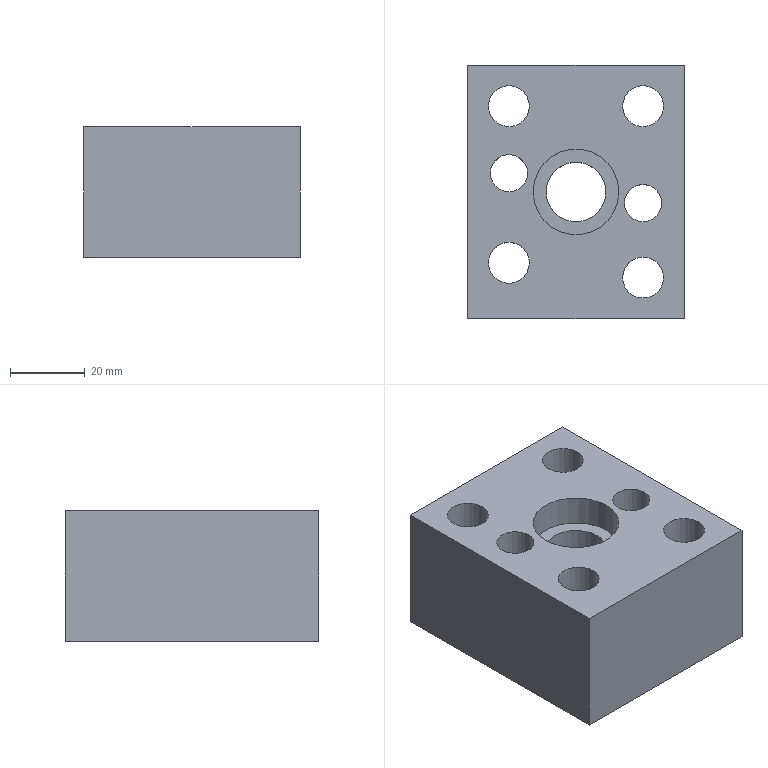Part | NX | features solid 2 | 1 solid | 27 faces | box 58 x 68 x 35 mm | volume 103779 mm3 | cylinder 14 | plane 13 | commonest cylinder face diameters 11 x6 17 x4 10 x2 16 x1 23 x1
STEP:
#1=CARTESIAN_POINT('',(1273.079,146.904,15.));
#2=VERTEX_POINT('',#1);
#3=CARTESIAN_POINT('',(1268.079,146.904,15.));
#4=DIRECTION('',(0.,0.,-1.));
#5=DIRECTION('',(1.,0.,0.));
#6=AXIS2_PLACEMENT_3D('',#3,#4,#5);
#7=CIRCLE('',#6,5.);
#8=EDGE_CURVE('',#2,#2,#7,.T.);
#9=ORIENTED_EDGE('',*,*,#8,.F.);
#10=EDGE_LOOP('',(#9));
#11=FACE_BOUND('',#10,.T.);
#12=CARTESIAN_POINT('',(1273.579,146.904,15.));
#13=VERTEX_POINT('',#12);
#14=CARTESIAN_POINT('',(1268.079,146.904,15.));
#15=DIRECTION('',(0.,0.,-1.));
#16=DIRECTION('',(1.,0.,0.));
#17=AXIS2_PLACEMENT_3D('',#14,#15,#16);
#18=CIRCLE('',#17,5.5);
#19=EDGE_CURVE('',#13,#13,#18,.T.);
#20=ORIENTED_EDGE('',*,*,#19,.T.);
#21=EDGE_LOOP('',(#20));
#22=FACE_BOUND('',#21,.T.);
#23=CARTESIAN_POINT('',(1266.894,137.78,15.));
#24=DIRECTION('',(0.,0.,1.));
#25=DIRECTION('',(1.,0.,0.));
#26=AXIS2_PLACEMENT_3D('',#23,#24,#25);
#27=PLANE('',#26);
#28=ADVANCED_FACE('',(#11,#22),#27,.F.);
#29=CARTESIAN_POINT('',(1273.079,146.904,40.));
#30=VERTEX_POINT('',#29);
#31=CARTESIAN_POINT('',(1268.079,146.904,40.));
#32=DIRECTION('',(0.,0.,-1.));
#33=DIRECTION('',(1.,0.,0.));
#34=AXIS2_PLACEMENT_3D('',#31,#32,#33);
#35=CIRCLE('',#34,5.);
#36=EDGE_CURVE('',#30,#30,#35,.T.);
#37=ORIENTED_EDGE('',*,*,#36,.F.);
#38=EDGE_LOOP('',(#37));
#39=FACE_BOUND('',#38,.T.);
#40=ORIENTED_EDGE('',*,*,#8,.T.);
#41=EDGE_LOOP('',(#40));
#42=FACE_BOUND('',#41,.T.);
#43=CARTESIAN_POINT('',(1268.079,146.904,40.));
#44=DIRECTION('',(0.,0.,1.));
#45=DIRECTION('',(1.,0.,0.));
#46=AXIS2_PLACEMENT_3D('',#43,#44,#45);
#47=CYLINDRICAL_SURFACE('',#46,5.);
#48=ADVANCED_FACE('',(#39,#42),#47,.F.);
#49=ORIENTED_EDGE('',*,*,#19,.F.);
#50=EDGE_LOOP('',(#49));
#51=FACE_BOUND('',#50,.T.);
#52=CARTESIAN_POINT('',(1273.579,146.904,5.));
#53=VERTEX_POINT('',#52);
#54=CARTESIAN_POINT('',(1268.079,146.904,5.));
#55=DIRECTION('',(0.,0.,-1.));
#56=DIRECTION('',(1.,0.,0.));
#57=AXIS2_PLACEMENT_3D('',#54,#55,#56);
#58=CIRCLE('',#57,5.5);
#59=EDGE_CURVE('',#53,#53,#58,.F.);
#60=ORIENTED_EDGE('',*,*,#59,.F.);
#61=EDGE_LOOP('',(#60));
#62=FACE_BOUND('',#61,.T.);
#63=CARTESIAN_POINT('',(1268.079,146.904,5.));
#64=DIRECTION('',(0.,0.,1.));
#65=DIRECTION('',(1.,0.,0.));
#66=AXIS2_PLACEMENT_3D('',#63,#64,#65);
#67=CYLINDRICAL_SURFACE('',#66,5.5);
#68=ADVANCED_FACE('',(#51,#62),#67,.F.);
#69=CARTESIAN_POINT('',(1298.579,118.904,17.));
#70=VERTEX_POINT('',#69);
#71=CARTESIAN_POINT('',(1304.079,118.904,17.));
#72=DIRECTION('',(0.,0.,1.));
#73=DIRECTION('',(-1.,0.,0.));
#74=AXIS2_PLACEMENT_3D('',#71,#72,#73);
#75=CIRCLE('',#74,5.5);
#76=EDGE_CURVE('',#70,#70,#75,.F.);
#77=ORIENTED_EDGE('',*,*,#76,.F.);
#78=EDGE_LOOP('',(#77));
#79=FACE_BOUND('',#78,.T.);
#80=CARTESIAN_POINT('',(1295.579,118.904,17.));
#81=VERTEX_POINT('',#80);
#82=CARTESIAN_POINT('',(1304.079,118.904,17.));
#83=DIRECTION('',(0.,0.,1.));
#84=DIRECTION('',(-1.,0.,0.));
#85=AXIS2_PLACEMENT_3D('',#82,#83,#84);
#86=CIRCLE('',#85,8.5);
#87=EDGE_CURVE('',#81,#81,#86,.F.);
#88=ORIENTED_EDGE('',*,*,#87,.T.);
#89=EDGE_LOOP('',(#88));
#90=FACE_BOUND('',#89,.T.);
#91=CARTESIAN_POINT('',(1304.074,120.57,17.));
#92=DIRECTION('',(0.,0.,1.));
#93=DIRECTION('',(-1.,0.,0.));
#94=AXIS2_PLACEMENT_3D('',#91,#92,#93);
#95=PLANE('',#94);
#96=ADVANCED_FACE('',(#79,#90),#95,.F.);
#97=CARTESIAN_POINT('',(1298.579,164.904,17.));
#98=VERTEX_POINT('',#97);
#99=CARTESIAN_POINT('',(1304.079,164.904,17.));
#100=DIRECTION('',(0.,0.,-1.));
#101=DIRECTION('',(-1.,0.,0.));
#102=AXIS2_PLACEMENT_3D('',#99,#100,#101);
#103=CIRCLE('',#102,5.5);
#104=EDGE_CURVE('',#98,#98,#103,.T.);
#105=ORIENTED_EDGE('',*,*,#104,.F.);
#106=EDGE_LOOP('',(#105));
#107=FACE_BOUND('',#106,.T.);
#108=CARTESIAN_POINT('',(1295.579,164.904,17.));
#109=VERTEX_POINT('',#108);
#110=CARTESIAN_POINT('',(1304.079,164.904,17.));
#111=DIRECTION('',(0.,0.,-1.));
#112=DIRECTION('',(-1.,0.,0.));
#113=AXIS2_PLACEMENT_3D('',#110,#111,#112);
#114=CIRCLE('',#113,8.5);
#115=EDGE_CURVE('',#109,#109,#114,.T.);
#116=ORIENTED_EDGE('',*,*,#115,.T.);
#117=EDGE_LOOP('',(#116));
#118=FACE_BOUND('',#117,.T.);
#119=CARTESIAN_POINT('',(1304.074,163.238,17.));
#120=DIRECTION('',(0.,0.,1.));
#121=DIRECTION('',(-1.,0.,0.));
#122=AXIS2_PLACEMENT_3D('',#119,#120,#121);
#123=PLANE('',#122);
#124=ADVANCED_FACE('',(#107,#118),#123,.F.);
#125=CARTESIAN_POINT('',(1273.579,164.904,17.));
#126=VERTEX_POINT('',#125);
#127=CARTESIAN_POINT('',(1268.079,164.904,17.));
#128=DIRECTION('',(0.,0.,1.));
#129=DIRECTION('',(1.,0.,0.));
#130=AXIS2_PLACEMENT_3D('',#127,#128,#129);
#131=CIRCLE('',#130,5.5);
#132=EDGE_CURVE('',#126,#126,#131,.F.);
#133=ORIENTED_EDGE('',*,*,#132,.F.);
#134=EDGE_LOOP('',(#133));
#135=FACE_BOUND('',#134,.T.);
#136=CARTESIAN_POINT('',(1276.579,164.904,17.));
#137=VERTEX_POINT('',#136);
#138=CARTESIAN_POINT('',(1268.079,164.904,17.));
#139=DIRECTION('',(0.,0.,1.));
#140=DIRECTION('',(1.,0.,0.));
#141=AXIS2_PLACEMENT_3D('',#138,#139,#140);
#142=CIRCLE('',#141,8.5);
#143=EDGE_CURVE('',#137,#137,#142,.F.);
#144=ORIENTED_EDGE('',*,*,#143,.T.);
#145=EDGE_LOOP('',(#144));
#146=FACE_BOUND('',#145,.T.);
#147=CARTESIAN_POINT('',(1268.083,163.238,17.));
#148=DIRECTION('',(0.,0.,1.));
#149=DIRECTION('',(1.,0.,0.));
#150=AXIS2_PLACEMENT_3D('',#147,#148,#149);
#151=PLANE('',#150);
#152=ADVANCED_FACE('',(#135,#146),#151,.F.);
#153=CARTESIAN_POINT('',(1273.579,122.904,17.));
#154=VERTEX_POINT('',#153);
#155=CARTESIAN_POINT('',(1268.079,122.904,17.));
#156=DIRECTION('',(0.,0.,-1.));
#157=DIRECTION('',(1.,0.,0.));
#158=AXIS2_PLACEMENT_3D('',#155,#156,#157);
#159=CIRCLE('',#158,5.5);
#160=EDGE_CURVE('',#154,#154,#159,.T.);
#161=ORIENTED_EDGE('',*,*,#160,.F.);
#162=EDGE_LOOP('',(#161));
#163=FACE_BOUND('',#162,.T.);
#164=CARTESIAN_POINT('',(1276.579,122.904,17.));
#165=VERTEX_POINT('',#164);
#166=CARTESIAN_POINT('',(1268.079,122.904,17.));
#167=DIRECTION('',(0.,0.,-1.));
#168=DIRECTION('',(1.,0.,0.));
#169=AXIS2_PLACEMENT_3D('',#166,#167,#168);
#170=CIRCLE('',#169,8.5);
#171=EDGE_CURVE('',#165,#165,#170,.T.);
#172=ORIENTED_EDGE('',*,*,#171,.T.);
#173=EDGE_LOOP('',(#172));
#174=FACE_BOUND('',#173,.T.);
#175=CARTESIAN_POINT('',(1268.083,124.57,17.));
#176=DIRECTION('',(0.,0.,1.));
#177=DIRECTION('',(1.,0.,0.));
#178=AXIS2_PLACEMENT_3D('',#175,#176,#177);
#179=PLANE('',#178);
#180=ADVANCED_FACE('',(#163,#174),#179,.F.);
#181=CARTESIAN_POINT('',(1299.079,138.904,15.));
#182=VERTEX_POINT('',#181);
#183=CARTESIAN_POINT('',(1304.079,138.904,15.));
#184=DIRECTION('',(0.,0.,1.));
#185=DIRECTION('',(-1.,0.,0.));
#186=AXIS2_PLACEMENT_3D('',#183,#184,#185);
#187=CIRCLE('',#186,5.);
#188=EDGE_CURVE('',#182,#182,#187,.F.);
#189=ORIENTED_EDGE('',*,*,#188,.F.);
#190=EDGE_LOOP('',(#189));
#191=FACE_BOUND('',#190,.T.);
#192=CARTESIAN_POINT('',(1298.579,138.904,15.));
#193=VERTEX_POINT('',#192);
#194=CARTESIAN_POINT('',(1304.079,138.904,15.));
#195=DIRECTION('',(0.,0.,1.));
#196=DIRECTION('',(-1.,0.,0.));
#197=AXIS2_PLACEMENT_3D('',#194,#195,#196);
#198=CIRCLE('',#197,5.5);
#199=EDGE_CURVE('',#193,#193,#198,.F.);
#200=ORIENTED_EDGE('',*,*,#199,.T.);
#201=EDGE_LOOP('',(#200));
#202=FACE_BOUND('',#201,.T.);
#203=CARTESIAN_POINT('',(1305.263,137.78,15.));
#204=DIRECTION('',(0.,0.,1.));
#205=DIRECTION('',(-1.,0.,0.));
#206=AXIS2_PLACEMENT_3D('',#203,#204,#205);
#207=PLANE('',#206);
#208=ADVANCED_FACE('',(#191,#202),#207,.F.);
#209=CARTESIAN_POINT('',(1315.079,175.904,5.));
#210=VERTEX_POINT('',#209);
#211=CARTESIAN_POINT('',(1315.079,175.904,40.));
#212=VERTEX_POINT('',#211);
#213=CARTESIAN_POINT('',(1315.079,175.904,12.));
#214=DIRECTION('',(0.,0.,1.));
#215=VECTOR('',#214,1000.);
#216=LINE('',#213,#215);
#217=EDGE_CURVE('',#210,#212,#216,.T.);
#218=ORIENTED_EDGE('',*,*,#217,.T.);
#219=CARTESIAN_POINT('',(1315.079,107.904,40.));
#220=VERTEX_POINT('',#219);
#221=CARTESIAN_POINT('',(1315.079,141.904,40.));
#222=DIRECTION('',(0.,1.,0.));
#223=VECTOR('',#222,1000.);
#224=LINE('',#221,#223);
#225=EDGE_CURVE('',#212,#220,#224,.F.);
#226=ORIENTED_EDGE('',*,*,#225,.T.);
#227=CARTESIAN_POINT('',(1315.079,107.904,5.));
#228=VERTEX_POINT('',#227);
#229=CARTESIAN_POINT('',(1315.079,107.904,12.));
#230=DIRECTION('',(0.,0.,1.));
#231=VECTOR('',#230,1000.);
#232=LINE('',#229,#231);
#233=EDGE_CURVE('',#228,#220,#232,.T.);
#234=ORIENTED_EDGE('',*,*,#233,.F.);
#235=CARTESIAN_POINT('',(1315.079,141.904,5.));
#236=DIRECTION('',(0.,1.,0.));
#237=VECTOR('',#236,1000.);
#238=LINE('',#235,#237);
#239=EDGE_CURVE('',#228,#210,#238,.T.);
#240=ORIENTED_EDGE('',*,*,#239,.T.);
#241=EDGE_LOOP('',(#218,#226,#234,#240));
#242=FACE_BOUND('',#241,.T.);
#243=CARTESIAN_POINT('',(1315.079,141.904,12.));
#244=DIRECTION('',(1.,0.,0.));
#245=DIRECTION('',(0.,0.,1.));
#246=AXIS2_PLACEMENT_3D('',#243,#244,#245);
#247=PLANE('',#246);
#248=ADVANCED_FACE('',(#242),#247,.T.);
#249=ORIENTED_EDGE('',*,*,#233,.T.);
#250=CARTESIAN_POINT('',(1257.079,107.904,40.));
#251=VERTEX_POINT('',#250);
#252=CARTESIAN_POINT('',(1286.079,107.904,40.));
#253=DIRECTION('',(1.,0.,0.));
#254=VECTOR('',#253,1000.);
#255=LINE('',#252,#254);
#256=EDGE_CURVE('',#220,#251,#255,.F.);
#257=ORIENTED_EDGE('',*,*,#256,.T.);
#258=CARTESIAN_POINT('',(1257.079,107.904,5.));
#259=VERTEX_POINT('',#258);
#260=CARTESIAN_POINT('',(1257.079,107.904,12.));
#261=DIRECTION('',(0.,0.,1.));
#262=VECTOR('',#261,1000.);
#263=LINE('',#260,#262);
#264=EDGE_CURVE('',#259,#251,#263,.T.);
#265=ORIENTED_EDGE('',*,*,#264,.F.);
#266=CARTESIAN_POINT('',(1286.079,107.904,5.));
#267=DIRECTION('',(1.,0.,0.));
#268=VECTOR('',#267,1000.);
#269=LINE('',#266,#268);
#270=EDGE_CURVE('',#259,#228,#269,.T.);
#271=ORIENTED_EDGE('',*,*,#270,.T.);
#272=EDGE_LOOP('',(#249,#257,#265,#271));
#273=FACE_BOUND('',#272,.T.);
#274=CARTESIAN_POINT('',(1286.079,107.904,12.));
#275=DIRECTION('',(0.,-1.,0.));
#276=DIRECTION('',(0.,0.,1.));
#277=AXIS2_PLACEMENT_3D('',#274,#275,#276);
#278=PLANE('',#277);
#279=ADVANCED_FACE('',(#273),#278,.T.);
#280=CARTESIAN_POINT('',(1257.079,175.904,5.));
#281=VERTEX_POINT('',#280);
#282=CARTESIAN_POINT('',(1257.079,141.904,5.));
#283=DIRECTION('',(0.,-1.,0.));
#284=VECTOR('',#283,1000.);
#285=LINE('',#282,#284);
#286=EDGE_CURVE('',#281,#259,#285,.T.);
#287=ORIENTED_EDGE('',*,*,#286,.T.);
#288=ORIENTED_EDGE('',*,*,#264,.T.);
#289=CARTESIAN_POINT('',(1257.079,175.904,40.));
#290=VERTEX_POINT('',#289);
#291=CARTESIAN_POINT('',(1257.079,141.904,40.));
#292=DIRECTION('',(0.,-1.,0.));
#293=VECTOR('',#292,1000.);
#294=LINE('',#291,#293);
#295=EDGE_CURVE('',#251,#290,#294,.F.);
#296=ORIENTED_EDGE('',*,*,#295,.T.);
#297=CARTESIAN_POINT('',(1257.079,175.904,12.));
#298=DIRECTION('',(0.,0.,1.));
#299=VECTOR('',#298,1000.);
#300=LINE('',#297,#299);
#301=EDGE_CURVE('',#281,#290,#300,.T.);
#302=ORIENTED_EDGE('',*,*,#301,.F.);
#303=EDGE_LOOP('',(#287,#288,#296,#302));
#304=FACE_BOUND('',#303,.T.);
#305=CARTESIAN_POINT('',(1257.079,141.904,12.));
#306=DIRECTION('',(-1.,0.,0.));
#307=DIRECTION('',(0.,0.,-1.));
#308=AXIS2_PLACEMENT_3D('',#305,#306,#307);
#309=PLANE('',#308);
#310=ADVANCED_FACE('',(#304),#309,.T.);
#311=ORIENTED_EDGE('',*,*,#301,.T.);
#312=CARTESIAN_POINT('',(1286.079,175.904,40.));
#313=DIRECTION('',(-1.,0.,0.));
#314=VECTOR('',#313,1000.);
#315=LINE('',#312,#314);
#316=EDGE_CURVE('',#290,#212,#315,.F.);
#317=ORIENTED_EDGE('',*,*,#316,.T.);
#318=ORIENTED_EDGE('',*,*,#217,.F.);
#319=CARTESIAN_POINT('',(1286.079,175.904,5.));
#320=DIRECTION('',(-1.,0.,0.));
#321=VECTOR('',#320,1000.);
#322=LINE('',#319,#321);
#323=EDGE_CURVE('',#210,#281,#322,.T.);
#324=ORIENTED_EDGE('',*,*,#323,.T.);
#325=EDGE_LOOP('',(#311,#317,#318,#324));
#326=FACE_BOUND('',#325,.T.);
#327=CARTESIAN_POINT('',(1286.079,175.904,12.));
#328=DIRECTION('',(0.,1.,0.));
#329=DIRECTION('',(0.,0.,-1.));
#330=AXIS2_PLACEMENT_3D('',#327,#328,#329);
#331=PLANE('',#330);
#332=ADVANCED_FACE('',(#326),#331,.T.);
#333=CARTESIAN_POINT('',(1298.579,118.904,40.));
#334=VERTEX_POINT('',#333);
#335=CARTESIAN_POINT('',(1304.079,118.904,40.));
#336=DIRECTION('',(0.,0.,1.));
#337=DIRECTION('',(-1.,0.,0.));
#338=AXIS2_PLACEMENT_3D('',#335,#336,#337);
#339=CIRCLE('',#338,5.5);
#340=EDGE_CURVE('',#334,#334,#339,.T.);
#341=ORIENTED_EDGE('',*,*,#340,.T.);
#342=EDGE_LOOP('',(#341));
#343=FACE_BOUND('',#342,.T.);
#344=ORIENTED_EDGE('',*,*,#76,.T.);
#345=EDGE_LOOP('',(#344));
#346=FACE_BOUND('',#345,.T.);
#347=CARTESIAN_POINT('',(1304.079,118.904,40.));
#348=DIRECTION('',(0.,0.,1.));
#349=DIRECTION('',(-1.,0.,0.));
#350=AXIS2_PLACEMENT_3D('',#347,#348,#349);
#351=CYLINDRICAL_SURFACE('',#350,5.5);
#352=ADVANCED_FACE('',(#343,#346),#351,.F.);
#353=CARTESIAN_POINT('',(1298.579,164.904,40.));
#354=VERTEX_POINT('',#353);
#355=CARTESIAN_POINT('',(1304.079,164.904,40.));
#356=DIRECTION('',(0.,0.,-1.));
#357=DIRECTION('',(-1.,0.,0.));
#358=AXIS2_PLACEMENT_3D('',#355,#356,#357);
#359=CIRCLE('',#358,5.5);
#360=EDGE_CURVE('',#354,#354,#359,.T.);
#361=ORIENTED_EDGE('',*,*,#360,.F.);
#362=EDGE_LOOP('',(#361));
#363=FACE_BOUND('',#362,.T.);
#364=ORIENTED_EDGE('',*,*,#104,.T.);
#365=EDGE_LOOP('',(#364));
#366=FACE_BOUND('',#365,.T.);
#367=CARTESIAN_POINT('',(1304.079,164.904,40.));
#368=DIRECTION('',(0.,0.,1.));
#369=DIRECTION('',(-1.,0.,0.));
#370=AXIS2_PLACEMENT_3D('',#367,#368,#369);
#371=CYLINDRICAL_SURFACE('',#370,5.5);
#372=ADVANCED_FACE('',(#363,#366),#371,.F.);
#373=CARTESIAN_POINT('',(1273.579,164.904,40.));
#374=VERTEX_POINT('',#373);
#375=CARTESIAN_POINT('',(1268.079,164.904,40.));
#376=DIRECTION('',(0.,0.,1.));
#377=DIRECTION('',(1.,0.,0.));
#378=AXIS2_PLACEMENT_3D('',#375,#376,#377);
#379=CIRCLE('',#378,5.5);
#380=EDGE_CURVE('',#374,#374,#379,.F.);
#381=ORIENTED_EDGE('',*,*,#380,.F.);
#382=EDGE_LOOP('',(#381));
#383=FACE_BOUND('',#382,.T.);
#384=ORIENTED_EDGE('',*,*,#132,.T.);
#385=EDGE_LOOP('',(#384));
#386=FACE_BOUND('',#385,.T.);
#387=CARTESIAN_POINT('',(1268.079,164.904,40.));
#388=DIRECTION('',(0.,0.,1.));
#389=DIRECTION('',(1.,0.,0.));
#390=AXIS2_PLACEMENT_3D('',#387,#388,#389);
#391=CYLINDRICAL_SURFACE('',#390,5.5);
#392=ADVANCED_FACE('',(#383,#386),#391,.F.);
#393=CARTESIAN_POINT('',(1273.579,122.904,40.));
#394=VERTEX_POINT('',#393);
#395=CARTESIAN_POINT('',(1268.079,122.904,40.));
#396=DIRECTION('',(0.,0.,-1.));
#397=DIRECTION('',(1.,0.,0.));
#398=AXIS2_PLACEMENT_3D('',#395,#396,#397);
#399=CIRCLE('',#398,5.5);
#400=EDGE_CURVE('',#394,#394,#399,.T.);
#401=ORIENTED_EDGE('',*,*,#400,.F.);
#402=EDGE_LOOP('',(#401));
#403=FACE_BOUND('',#402,.T.);
#404=ORIENTED_EDGE('',*,*,#160,.T.);
#405=EDGE_LOOP('',(#404));
#406=FACE_BOUND('',#405,.T.);
#407=CARTESIAN_POINT('',(1268.079,122.904,40.));
#408=DIRECTION('',(0.,0.,1.));
#409=DIRECTION('',(1.,0.,0.));
#410=AXIS2_PLACEMENT_3D('',#407,#408,#409);
#411=CYLINDRICAL_SURFACE('',#410,5.5);
#412=ADVANCED_FACE('',(#403,#406),#411,.F.);
#413=CARTESIAN_POINT('',(1299.079,138.904,40.));
#414=VERTEX_POINT('',#413);
#415=CARTESIAN_POINT('',(1304.079,138.904,40.));
#416=DIRECTION('',(0.,0.,1.));
#417=DIRECTION('',(-1.,0.,0.));
#418=AXIS2_PLACEMENT_3D('',#415,#416,#417);
#419=CIRCLE('',#418,5.);
#420=EDGE_CURVE('',#414,#414,#419,.T.);
#421=ORIENTED_EDGE('',*,*,#420,.T.);
#422=EDGE_LOOP('',(#421));
#423=FACE_BOUND('',#422,.T.);
#424=ORIENTED_EDGE('',*,*,#188,.T.);
#425=EDGE_LOOP('',(#424));
#426=FACE_BOUND('',#425,.T.);
#427=CARTESIAN_POINT('',(1304.079,138.904,40.));
#428=DIRECTION('',(0.,0.,1.));
#429=DIRECTION('',(-1.,0.,0.));
#430=AXIS2_PLACEMENT_3D('',#427,#428,#429);
#431=CYLINDRICAL_SURFACE('',#430,5.);
#432=ADVANCED_FACE('',(#423,#426),#431,.F.);
#433=CARTESIAN_POINT('',(1274.579,141.904,40.));
#434=VERTEX_POINT('',#433);
#435=CARTESIAN_POINT('',(1286.079,141.904,40.));
#436=DIRECTION('',(0.,0.,1.));
#437=DIRECTION('',(-1.,0.,0.));
#438=AXIS2_PLACEMENT_3D('',#435,#436,#437);
#439=CIRCLE('',#438,11.5);
#440=EDGE_CURVE('',#434,#434,#439,.F.);
#441=ORIENTED_EDGE('',*,*,#440,.T.);
#442=EDGE_LOOP('',(#441));
#443=FACE_BOUND('',#442,.T.);
#444=ORIENTED_EDGE('',*,*,#36,.T.);
#445=EDGE_LOOP('',(#444));
#446=FACE_BOUND('',#445,.T.);
#447=ORIENTED_EDGE('',*,*,#420,.F.);
#448=EDGE_LOOP('',(#447));
#449=FACE_BOUND('',#448,.T.);
#450=ORIENTED_EDGE('',*,*,#400,.T.);
#451=EDGE_LOOP('',(#450));
#452=FACE_BOUND('',#451,.T.);
#453=ORIENTED_EDGE('',*,*,#380,.T.);
#454=EDGE_LOOP('',(#453));
#455=FACE_BOUND('',#454,.T.);
#456=ORIENTED_EDGE('',*,*,#360,.T.);
#457=EDGE_LOOP('',(#456));
#458=FACE_BOUND('',#457,.T.);
#459=ORIENTED_EDGE('',*,*,#340,.F.);
#460=EDGE_LOOP('',(#459));
#461=FACE_BOUND('',#460,.T.);
#462=ORIENTED_EDGE('',*,*,#316,.F.);
#463=ORIENTED_EDGE('',*,*,#295,.F.);
#464=ORIENTED_EDGE('',*,*,#256,.F.);
#465=ORIENTED_EDGE('',*,*,#225,.F.);
#466=EDGE_LOOP('',(#462,#463,#464,#465));
#467=FACE_BOUND('',#466,.T.);
#468=CARTESIAN_POINT('',(2087.158,0.000000688,40.));
#469=DIRECTION('',(0.,0.,-1.));
#470=DIRECTION('',(1.,0.,0.));
#471=AXIS2_PLACEMENT_3D('',#468,#469,#470);
#472=PLANE('',#471);
#473=ADVANCED_FACE('',(#443,#446,#449,#452,#455,#458,#461,#467),#472,.F.);
#474=ORIENTED_EDGE('',*,*,#87,.F.);
#475=EDGE_LOOP('',(#474));
#476=FACE_BOUND('',#475,.T.);
#477=CARTESIAN_POINT('',(1295.579,118.904,5.));
#478=VERTEX_POINT('',#477);
#479=CARTESIAN_POINT('',(1304.079,118.904,5.));
#480=DIRECTION('',(0.,0.,1.));
#481=DIRECTION('',(-1.,0.,0.));
#482=AXIS2_PLACEMENT_3D('',#479,#480,#481);
#483=CIRCLE('',#482,8.5);
#484=EDGE_CURVE('',#478,#478,#483,.T.);
#485=ORIENTED_EDGE('',*,*,#484,.F.);
#486=EDGE_LOOP('',(#485));
#487=FACE_BOUND('',#486,.T.);
#488=CARTESIAN_POINT('',(1304.079,118.904,5.));
#489=DIRECTION('',(0.,0.,1.));
#490=DIRECTION('',(-1.,0.,0.));
#491=AXIS2_PLACEMENT_3D('',#488,#489,#490);
#492=CYLINDRICAL_SURFACE('',#491,8.5);
#493=ADVANCED_FACE('',(#476,#487),#492,.F.);
#494=ORIENTED_EDGE('',*,*,#115,.F.);
#495=EDGE_LOOP('',(#494));
#496=FACE_BOUND('',#495,.T.);
#497=CARTESIAN_POINT('',(1295.579,164.904,5.));
#498=VERTEX_POINT('',#497);
#499=CARTESIAN_POINT('',(1304.079,164.904,5.));
#500=DIRECTION('',(0.,0.,-1.));
#501=DIRECTION('',(-1.,0.,0.));
#502=AXIS2_PLACEMENT_3D('',#499,#500,#501);
#503=CIRCLE('',#502,8.5);
#504=EDGE_CURVE('',#498,#498,#503,.F.);
#505=ORIENTED_EDGE('',*,*,#504,.F.);
#506=EDGE_LOOP('',(#505));
#507=FACE_BOUND('',#506,.T.);
#508=CARTESIAN_POINT('',(1304.079,164.904,5.));
#509=DIRECTION('',(0.,0.,1.));
#510=DIRECTION('',(-1.,0.,0.));
#511=AXIS2_PLACEMENT_3D('',#508,#509,#510);
#512=CYLINDRICAL_SURFACE('',#511,8.5);
#513=ADVANCED_FACE('',(#496,#507),#512,.F.);
#514=ORIENTED_EDGE('',*,*,#143,.F.);
#515=EDGE_LOOP('',(#514));
#516=FACE_BOUND('',#515,.T.);
#517=CARTESIAN_POINT('',(1276.579,164.904,5.));
#518=VERTEX_POINT('',#517);
#519=CARTESIAN_POINT('',(1268.079,164.904,5.));
#520=DIRECTION('',(0.,0.,1.));
#521=DIRECTION('',(1.,0.,0.));
#522=AXIS2_PLACEMENT_3D('',#519,#520,#521);
#523=CIRCLE('',#522,8.5);
#524=EDGE_CURVE('',#518,#518,#523,.T.);
#525=ORIENTED_EDGE('',*,*,#524,.F.);
#526=EDGE_LOOP('',(#525));
#527=FACE_BOUND('',#526,.T.);
#528=CARTESIAN_POINT('',(1268.079,164.904,5.));
#529=DIRECTION('',(0.,0.,1.));
#530=DIRECTION('',(1.,0.,0.));
#531=AXIS2_PLACEMENT_3D('',#528,#529,#530);
#532=CYLINDRICAL_SURFACE('',#531,8.5);
#533=ADVANCED_FACE('',(#516,#527),#532,.F.);
#534=ORIENTED_EDGE('',*,*,#171,.F.);
#535=EDGE_LOOP('',(#534));
#536=FACE_BOUND('',#535,.T.);
#537=CARTESIAN_POINT('',(1276.579,122.904,5.));
#538=VERTEX_POINT('',#537);
#539=CARTESIAN_POINT('',(1268.079,122.904,5.));
#540=DIRECTION('',(0.,0.,-1.));
#541=DIRECTION('',(1.,0.,0.));
#542=AXIS2_PLACEMENT_3D('',#539,#540,#541);
#543=CIRCLE('',#542,8.5);
#544=EDGE_CURVE('',#538,#538,#543,.F.);
#545=ORIENTED_EDGE('',*,*,#544,.F.);
#546=EDGE_LOOP('',(#545));
#547=FACE_BOUND('',#546,.T.);
#548=CARTESIAN_POINT('',(1268.079,122.904,5.));
#549=DIRECTION('',(0.,0.,1.));
#550=DIRECTION('',(1.,0.,0.));
#551=AXIS2_PLACEMENT_3D('',#548,#549,#550);
#552=CYLINDRICAL_SURFACE('',#551,8.5);
#553=ADVANCED_FACE('',(#536,#547),#552,.F.);
#554=ORIENTED_EDGE('',*,*,#199,.F.);
#555=EDGE_LOOP('',(#554));
#556=FACE_BOUND('',#555,.T.);
#557=CARTESIAN_POINT('',(1298.579,138.904,5.));
#558=VERTEX_POINT('',#557);
#559=CARTESIAN_POINT('',(1304.079,138.904,5.));
#560=DIRECTION('',(0.,0.,1.));
#561=DIRECTION('',(-1.,0.,0.));
#562=AXIS2_PLACEMENT_3D('',#559,#560,#561);
#563=CIRCLE('',#562,5.5);
#564=EDGE_CURVE('',#558,#558,#563,.T.);
#565=ORIENTED_EDGE('',*,*,#564,.F.);
#566=EDGE_LOOP('',(#565));
#567=FACE_BOUND('',#566,.T.);
#568=CARTESIAN_POINT('',(1304.079,138.904,5.));
#569=DIRECTION('',(0.,0.,1.));
#570=DIRECTION('',(-1.,0.,0.));
#571=AXIS2_PLACEMENT_3D('',#568,#569,#570);
#572=CYLINDRICAL_SURFACE('',#571,5.5);
#573=ADVANCED_FACE('',(#556,#567),#572,.F.);
#574=CARTESIAN_POINT('',(1294.079,141.904,5.));
#575=VERTEX_POINT('',#574);
#576=CARTESIAN_POINT('',(1286.079,141.904,5.));
#577=DIRECTION('',(0.,0.,-1.));
#578=DIRECTION('',(1.,0.,0.));
#579=AXIS2_PLACEMENT_3D('',#576,#577,#578);
#580=CIRCLE('',#579,8.);
#581=EDGE_CURVE('',#575,#575,#580,.T.);
#582=ORIENTED_EDGE('',*,*,#581,.F.);
#583=EDGE_LOOP('',(#582));
#584=FACE_BOUND('',#583,.T.);
#585=ORIENTED_EDGE('',*,*,#59,.T.);
#586=EDGE_LOOP('',(#585));
#587=FACE_BOUND('',#586,.T.);
#588=ORIENTED_EDGE('',*,*,#564,.T.);
#589=EDGE_LOOP('',(#588));
#590=FACE_BOUND('',#589,.T.);
#591=ORIENTED_EDGE('',*,*,#544,.T.);
#592=EDGE_LOOP('',(#591));
#593=FACE_BOUND('',#592,.T.);
#594=ORIENTED_EDGE('',*,*,#524,.T.);
#595=EDGE_LOOP('',(#594));
#596=FACE_BOUND('',#595,.T.);
#597=ORIENTED_EDGE('',*,*,#504,.T.);
#598=EDGE_LOOP('',(#597));
#599=FACE_BOUND('',#598,.T.);
#600=ORIENTED_EDGE('',*,*,#484,.T.);
#601=EDGE_LOOP('',(#600));
#602=FACE_BOUND('',#601,.T.);
#603=ORIENTED_EDGE('',*,*,#286,.F.);
#604=ORIENTED_EDGE('',*,*,#323,.F.);
#605=ORIENTED_EDGE('',*,*,#239,.F.);
#606=ORIENTED_EDGE('',*,*,#270,.F.);
#607=EDGE_LOOP('',(#603,#604,#605,#606));
#608=FACE_BOUND('',#607,.T.);
#609=CARTESIAN_POINT('',(1286.079,141.904,5.));
#610=DIRECTION('',(0.,0.,-1.));
#611=DIRECTION('',(1.,0.,0.));
#612=AXIS2_PLACEMENT_3D('',#609,#610,#611);
#613=PLANE('',#612);
#614=ADVANCED_FACE('',(#584,#587,#590,#593,#596,#599,#602,#608),#613,.T.);
#615=ORIENTED_EDGE('',*,*,#581,.T.);
#616=EDGE_LOOP('',(#615));
#617=FACE_BOUND('',#616,.T.);
#618=CARTESIAN_POINT('',(1278.079,141.904,31.8));
#619=VERTEX_POINT('',#618);
#620=CARTESIAN_POINT('',(1286.079,141.904,31.8));
#621=DIRECTION('',(0.,0.,-1.));
#622=DIRECTION('',(-1.,0.,0.));
#623=AXIS2_PLACEMENT_3D('',#620,#621,#622);
#624=CIRCLE('',#623,8.);
#625=EDGE_CURVE('',#619,#619,#624,.T.);
#626=ORIENTED_EDGE('',*,*,#625,.F.);
#627=EDGE_LOOP('',(#626));
#628=FACE_BOUND('',#627,.T.);
#629=CARTESIAN_POINT('',(1286.079,141.904,40.));
#630=DIRECTION('',(0.,0.,-1.));
#631=DIRECTION('',(1.,0.,0.));
#632=AXIS2_PLACEMENT_3D('',#629,#630,#631);
#633=CYLINDRICAL_SURFACE('',#632,8.);
#634=ADVANCED_FACE('',(#617,#628),#633,.F.);
#635=CARTESIAN_POINT('',(1274.579,141.904,31.8));
#636=VERTEX_POINT('',#635);
#637=CARTESIAN_POINT('',(1286.079,141.904,31.8));
#638=DIRECTION('',(0.,0.,1.));
#639=DIRECTION('',(-1.,0.,0.));
#640=AXIS2_PLACEMENT_3D('',#637,#638,#639);
#641=CIRCLE('',#640,11.5);
#642=EDGE_CURVE('',#636,#636,#641,.T.);
#643=ORIENTED_EDGE('',*,*,#642,.F.);
#644=EDGE_LOOP('',(#643));
#645=FACE_BOUND('',#644,.T.);
#646=ORIENTED_EDGE('',*,*,#440,.F.);
#647=EDGE_LOOP('',(#646));
#648=FACE_BOUND('',#647,.T.);
#649=CARTESIAN_POINT('',(1286.079,141.904,40.));
#650=DIRECTION('',(0.,0.,-1.));
#651=DIRECTION('',(1.,0.,0.));
#652=AXIS2_PLACEMENT_3D('',#649,#650,#651);
#653=CYLINDRICAL_SURFACE('',#652,11.5);
#654=ADVANCED_FACE('',(#645,#648),#653,.F.);
#655=ORIENTED_EDGE('',*,*,#642,.T.);
#656=EDGE_LOOP('',(#655));
#657=FACE_BOUND('',#656,.T.);
#658=ORIENTED_EDGE('',*,*,#625,.T.);
#659=EDGE_LOOP('',(#658));
#660=FACE_BOUND('',#659,.T.);
#661=CARTESIAN_POINT('',(2087.158,0.000000688,31.8));
#662=DIRECTION('',(0.,0.,-1.));
#663=DIRECTION('',(1.,0.,0.));
#664=AXIS2_PLACEMENT_3D('',#661,#662,#663);
#665=PLANE('',#664);
#666=ADVANCED_FACE('',(#657,#660),#665,.F.);
#667=CLOSED_SHELL('',(#28,#48,#68,#96,#124,#152,#180,#208,#248,#279,#310,#332,#352,#372,#392,#412,#432,#473,#493,#513,#533,#553,#573,#614,#634,#654,#666));
#668=MANIFOLD_SOLID_BREP('',#667);
#669=(LENGTH_UNIT()NAMED_UNIT(*)SI_UNIT(.MILLI.,.METRE.));
#670=UNCERTAINTY_MEASURE_WITH_UNIT(LENGTH_MEASURE(0.00001),#669,'','');
#671=(NAMED_UNIT(*)PLANE_ANGLE_UNIT()SI_UNIT($,.RADIAN.));
#672=(NAMED_UNIT(*)SI_UNIT($,.STERADIAN.)SOLID_ANGLE_UNIT());
#673=(GEOMETRIC_REPRESENTATION_CONTEXT(3)GLOBAL_UNCERTAINTY_ASSIGNED_CONTEXT((#670))GLOBAL_UNIT_ASSIGNED_CONTEXT((#669,#671,#672))REPRESENTATION_CONTEXT('',''));
#674=ADVANCED_BREP_SHAPE_REPRESENTATION('',(#668),#673);